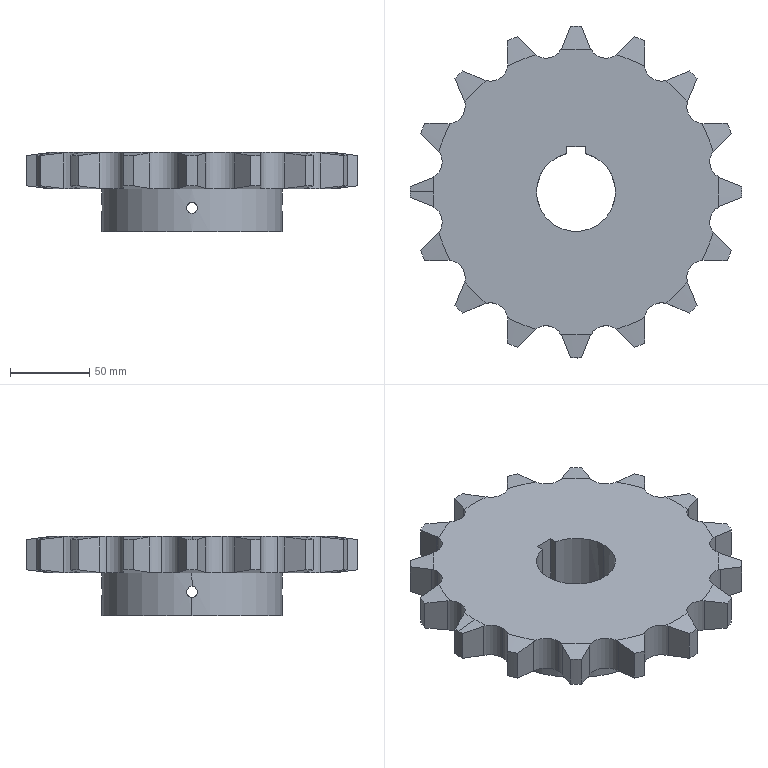Part | STEP file | 24A16T sprocket 2XG | 1 solid | 124 faces | box 210 x 210 x 50 mm | volume 809619 mm3 | cylinder 52 | plane 38 | cone 34 | commonest cylinder face diameters 22 x22 210 x17 6.8 x8 50 x3 114 x2